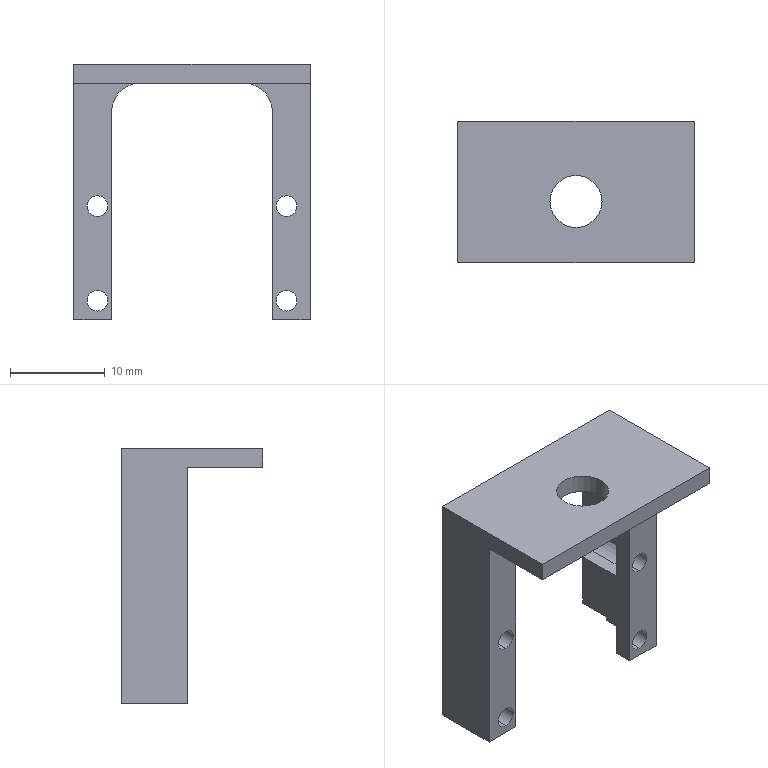Part | SolidWorks | features BaseBody 1 | 1 solid | 40 faces | box 25 x 15 x 27 mm | volume 1845 mm3 | plane 24 | cylinder 16 | commonest cylinder face diameters 2.2 x8 4 x4 5.5 x2 6 x2
STEP:
#1=CARTESIAN_POINT('',(9.75,-3.5,0.));
#2=VERTEX_POINT('',#1);
#3=CARTESIAN_POINT('',(15.25,-3.5,0.));
#4=VERTEX_POINT('',#3);
#5=CARTESIAN_POINT('',(12.5,-3.5,0.));
#6=DIRECTION('',(0.,0.,1.));
#7=DIRECTION('',(1.,0.,0.));
#8=AXIS2_PLACEMENT_3D('',#5,#6,#7);
#9=CIRCLE('',#8,2.75);
#10=EDGE_CURVE('',#2,#4,#9,.T.);
#11=ORIENTED_EDGE('',*,*,#10,.F.);
#12=CARTESIAN_POINT('',(9.75,-3.5,2.));
#13=VERTEX_POINT('',#12);
#14=CARTESIAN_POINT('',(9.75,-3.5,-13.));
#15=DIRECTION('',(0.,0.,1.));
#16=VECTOR('',#15,1000.);
#17=LINE('',#14,#16);
#18=EDGE_CURVE('',#2,#13,#17,.T.);
#19=ORIENTED_EDGE('',*,*,#18,.T.);
#20=CARTESIAN_POINT('',(15.25,-3.5,2.));
#21=VERTEX_POINT('',#20);
#22=CARTESIAN_POINT('',(12.5,-3.5,2.));
#23=DIRECTION('',(0.,0.,1.));
#24=DIRECTION('',(1.,0.,0.));
#25=AXIS2_PLACEMENT_3D('',#22,#23,#24);
#26=CIRCLE('',#25,2.75);
#27=EDGE_CURVE('',#13,#21,#26,.T.);
#28=ORIENTED_EDGE('',*,*,#27,.T.);
#29=CARTESIAN_POINT('',(15.25,-3.5,-13.));
#30=DIRECTION('',(0.,0.,1.));
#31=VECTOR('',#30,1000.);
#32=LINE('',#29,#31);
#33=EDGE_CURVE('',#4,#21,#32,.T.);
#34=ORIENTED_EDGE('',*,*,#33,.F.);
#35=EDGE_LOOP('',(#11,#19,#28,#34));
#36=FACE_OUTER_BOUND('',#35,.T.);
#37=CARTESIAN_POINT('',(12.5,-3.5,-13.));
#38=DIRECTION('',(0.,0.,1.));
#39=DIRECTION('',(1.,0.,0.));
#40=AXIS2_PLACEMENT_3D('',#37,#38,#39);
#41=CYLINDRICAL_SURFACE('',#40,2.75);
#42=ADVANCED_FACE('',(#36),#41,.F.);
#43=CARTESIAN_POINT('',(22.5,-2.,-21.9));
#44=VERTEX_POINT('',#43);
#45=CARTESIAN_POINT('',(22.5,-2.,-24.1));
#46=VERTEX_POINT('',#45);
#47=CARTESIAN_POINT('',(22.5,-2.,-23.));
#48=DIRECTION('',(0.,-1.,0.));
#49=DIRECTION('',(0.,0.,1.));
#50=AXIS2_PLACEMENT_3D('',#47,#48,#49);
#51=CIRCLE('',#50,1.1);
#52=EDGE_CURVE('',#44,#46,#51,.T.);
#53=ORIENTED_EDGE('',*,*,#52,.T.);
#54=CARTESIAN_POINT('',(22.5,0.,-24.1));
#55=VERTEX_POINT('',#54);
#56=CARTESIAN_POINT('',(22.5,-11.,-24.1));
#57=DIRECTION('',(0.,1.,0.));
#58=VECTOR('',#57,1000.);
#59=LINE('',#56,#58);
#60=EDGE_CURVE('',#46,#55,#59,.T.);
#61=ORIENTED_EDGE('',*,*,#60,.T.);
#62=CARTESIAN_POINT('',(22.5,0.,-21.9));
#63=VERTEX_POINT('',#62);
#64=CARTESIAN_POINT('',(22.5,0.,-23.));
#65=DIRECTION('',(0.,-1.,0.));
#66=DIRECTION('',(0.,0.,1.));
#67=AXIS2_PLACEMENT_3D('',#64,#65,#66);
#68=CIRCLE('',#67,1.1);
#69=EDGE_CURVE('',#63,#55,#68,.T.);
#70=ORIENTED_EDGE('',*,*,#69,.F.);
#71=CARTESIAN_POINT('',(22.5,-11.,-21.9));
#72=DIRECTION('',(0.,1.,0.));
#73=VECTOR('',#72,1000.);
#74=LINE('',#71,#73);
#75=EDGE_CURVE('',#44,#63,#74,.T.);
#76=ORIENTED_EDGE('',*,*,#75,.F.);
#77=EDGE_LOOP('',(#53,#61,#70,#76));
#78=FACE_OUTER_BOUND('',#77,.T.);
#79=CARTESIAN_POINT('',(22.5,-11.,-23.));
#80=DIRECTION('',(0.,1.,0.));
#81=DIRECTION('',(0.,0.,1.));
#82=AXIS2_PLACEMENT_3D('',#79,#80,#81);
#83=CYLINDRICAL_SURFACE('',#82,1.1);
#84=ADVANCED_FACE('',(#78),#83,.F.);
#85=CARTESIAN_POINT('',(22.5,-2.,-11.9));
#86=VERTEX_POINT('',#85);
#87=CARTESIAN_POINT('',(22.5,-2.,-14.1));
#88=VERTEX_POINT('',#87);
#89=CARTESIAN_POINT('',(22.5,-2.,-13.));
#90=DIRECTION('',(0.,-1.,0.));
#91=DIRECTION('',(0.,0.,1.));
#92=AXIS2_PLACEMENT_3D('',#89,#90,#91);
#93=CIRCLE('',#92,1.1);
#94=EDGE_CURVE('',#86,#88,#93,.T.);
#95=ORIENTED_EDGE('',*,*,#94,.T.);
#96=CARTESIAN_POINT('',(22.5,0.,-14.1));
#97=VERTEX_POINT('',#96);
#98=CARTESIAN_POINT('',(22.5,-11.,-14.1));
#99=DIRECTION('',(0.,1.,0.));
#100=VECTOR('',#99,1000.);
#101=LINE('',#98,#100);
#102=EDGE_CURVE('',#88,#97,#101,.T.);
#103=ORIENTED_EDGE('',*,*,#102,.T.);
#104=CARTESIAN_POINT('',(22.5,0.,-11.9));
#105=VERTEX_POINT('',#104);
#106=CARTESIAN_POINT('',(22.5,0.,-13.));
#107=DIRECTION('',(0.,-1.,0.));
#108=DIRECTION('',(0.,0.,1.));
#109=AXIS2_PLACEMENT_3D('',#106,#107,#108);
#110=CIRCLE('',#109,1.1);
#111=EDGE_CURVE('',#105,#97,#110,.T.);
#112=ORIENTED_EDGE('',*,*,#111,.F.);
#113=CARTESIAN_POINT('',(22.5,-11.,-11.9));
#114=DIRECTION('',(0.,1.,0.));
#115=VECTOR('',#114,1000.);
#116=LINE('',#113,#115);
#117=EDGE_CURVE('',#86,#105,#116,.T.);
#118=ORIENTED_EDGE('',*,*,#117,.F.);
#119=EDGE_LOOP('',(#95,#103,#112,#118));
#120=FACE_OUTER_BOUND('',#119,.T.);
#121=CARTESIAN_POINT('',(22.5,-11.,-13.));
#122=DIRECTION('',(0.,1.,0.));
#123=DIRECTION('',(0.,0.,1.));
#124=AXIS2_PLACEMENT_3D('',#121,#122,#123);
#125=CYLINDRICAL_SURFACE('',#124,1.1);
#126=ADVANCED_FACE('',(#120),#125,.F.);
#127=CARTESIAN_POINT('',(2.5,-2.,-11.9));
#128=VERTEX_POINT('',#127);
#129=CARTESIAN_POINT('',(2.5,-2.,-14.1));
#130=VERTEX_POINT('',#129);
#131=CARTESIAN_POINT('',(2.5,-2.,-13.));
#132=DIRECTION('',(0.,-1.,0.));
#133=DIRECTION('',(0.,0.,1.));
#134=AXIS2_PLACEMENT_3D('',#131,#132,#133);
#135=CIRCLE('',#134,1.1);
#136=EDGE_CURVE('',#128,#130,#135,.T.);
#137=ORIENTED_EDGE('',*,*,#136,.T.);
#138=CARTESIAN_POINT('',(2.5,0.,-14.1));
#139=VERTEX_POINT('',#138);
#140=CARTESIAN_POINT('',(2.5,-11.,-14.1));
#141=DIRECTION('',(0.,1.,0.));
#142=VECTOR('',#141,1000.);
#143=LINE('',#140,#142);
#144=EDGE_CURVE('',#130,#139,#143,.T.);
#145=ORIENTED_EDGE('',*,*,#144,.T.);
#146=CARTESIAN_POINT('',(2.5,0.,-11.9));
#147=VERTEX_POINT('',#146);
#148=CARTESIAN_POINT('',(2.5,0.,-13.));
#149=DIRECTION('',(0.,1.,0.));
#150=DIRECTION('',(0.,0.,1.));
#151=AXIS2_PLACEMENT_3D('',#148,#149,#150);
#152=CIRCLE('',#151,1.1);
#153=EDGE_CURVE('',#139,#147,#152,.T.);
#154=ORIENTED_EDGE('',*,*,#153,.T.);
#155=CARTESIAN_POINT('',(2.5,-11.,-11.9));
#156=DIRECTION('',(0.,1.,0.));
#157=VECTOR('',#156,1000.);
#158=LINE('',#155,#157);
#159=EDGE_CURVE('',#128,#147,#158,.T.);
#160=ORIENTED_EDGE('',*,*,#159,.F.);
#161=EDGE_LOOP('',(#137,#145,#154,#160));
#162=FACE_OUTER_BOUND('',#161,.T.);
#163=CARTESIAN_POINT('',(2.5,-11.,-13.));
#164=DIRECTION('',(0.,1.,0.));
#165=DIRECTION('',(0.,0.,1.));
#166=AXIS2_PLACEMENT_3D('',#163,#164,#165);
#167=CYLINDRICAL_SURFACE('',#166,1.1);
#168=ADVANCED_FACE('',(#162),#167,.F.);
#169=CARTESIAN_POINT('',(2.5,-2.,-21.9));
#170=VERTEX_POINT('',#169);
#171=CARTESIAN_POINT('',(2.5,-2.,-24.1));
#172=VERTEX_POINT('',#171);
#173=CARTESIAN_POINT('',(2.5,-2.,-23.));
#174=DIRECTION('',(0.,-1.,0.));
#175=DIRECTION('',(0.,0.,1.));
#176=AXIS2_PLACEMENT_3D('',#173,#174,#175);
#177=CIRCLE('',#176,1.1);
#178=EDGE_CURVE('',#170,#172,#177,.T.);
#179=ORIENTED_EDGE('',*,*,#178,.T.);
#180=CARTESIAN_POINT('',(2.5,0.,-24.1));
#181=VERTEX_POINT('',#180);
#182=CARTESIAN_POINT('',(2.5,-11.,-24.1));
#183=DIRECTION('',(0.,1.,0.));
#184=VECTOR('',#183,1000.);
#185=LINE('',#182,#184);
#186=EDGE_CURVE('',#172,#181,#185,.T.);
#187=ORIENTED_EDGE('',*,*,#186,.T.);
#188=CARTESIAN_POINT('',(2.5,0.,-21.9));
#189=VERTEX_POINT('',#188);
#190=CARTESIAN_POINT('',(2.5,0.,-23.));
#191=DIRECTION('',(0.,1.,0.));
#192=DIRECTION('',(0.,0.,1.));
#193=AXIS2_PLACEMENT_3D('',#190,#191,#192);
#194=CIRCLE('',#193,1.1);
#195=EDGE_CURVE('',#181,#189,#194,.T.);
#196=ORIENTED_EDGE('',*,*,#195,.T.);
#197=CARTESIAN_POINT('',(2.5,-11.,-21.9));
#198=DIRECTION('',(0.,1.,0.));
#199=VECTOR('',#198,1000.);
#200=LINE('',#197,#199);
#201=EDGE_CURVE('',#170,#189,#200,.T.);
#202=ORIENTED_EDGE('',*,*,#201,.F.);
#203=EDGE_LOOP('',(#179,#187,#196,#202));
#204=FACE_OUTER_BOUND('',#203,.T.);
#205=CARTESIAN_POINT('',(2.5,-11.,-23.));
#206=DIRECTION('',(0.,1.,0.));
#207=DIRECTION('',(0.,0.,1.));
#208=AXIS2_PLACEMENT_3D('',#205,#206,#207);
#209=CYLINDRICAL_SURFACE('',#208,1.1);
#210=ADVANCED_FACE('',(#204),#209,.F.);
#211=CARTESIAN_POINT('',(25.,5.,2.));
#212=VERTEX_POINT('',#211);
#213=CARTESIAN_POINT('',(25.,-10.,2.));
#214=VERTEX_POINT('',#213);
#215=CARTESIAN_POINT('',(25.,0.,2.));
#216=DIRECTION('',(0.,-1.,0.));
#217=VECTOR('',#216,1000.);
#218=LINE('',#215,#217);
#219=EDGE_CURVE('',#212,#214,#218,.T.);
#220=ORIENTED_EDGE('',*,*,#219,.F.);
#221=CARTESIAN_POINT('',(0.,5.,2.));
#222=VERTEX_POINT('',#221);
#223=CARTESIAN_POINT('',(0.,5.,2.));
#224=DIRECTION('',(1.,0.,0.));
#225=VECTOR('',#224,1000.);
#226=LINE('',#223,#225);
#227=EDGE_CURVE('',#222,#212,#226,.T.);
#228=ORIENTED_EDGE('',*,*,#227,.F.);
#229=CARTESIAN_POINT('',(0.,-10.,2.));
#230=VERTEX_POINT('',#229);
#231=CARTESIAN_POINT('',(0.,0.,2.));
#232=DIRECTION('',(0.,1.,0.));
#233=VECTOR('',#232,1000.);
#234=LINE('',#231,#233);
#235=EDGE_CURVE('',#230,#222,#234,.T.);
#236=ORIENTED_EDGE('',*,*,#235,.F.);
#237=CARTESIAN_POINT('',(0.,-10.,2.));
#238=DIRECTION('',(-1.,0.,0.));
#239=VECTOR('',#238,1000.);
#240=LINE('',#237,#239);
#241=EDGE_CURVE('',#214,#230,#240,.T.);
#242=ORIENTED_EDGE('',*,*,#241,.F.);
#243=EDGE_LOOP('',(#220,#228,#236,#242));
#244=FACE_OUTER_BOUND('',#243,.T.);
#245=CARTESIAN_POINT('',(12.5,-3.5,2.));
#246=DIRECTION('',(0.,0.,1.));
#247=DIRECTION('',(1.,0.,0.));
#248=AXIS2_PLACEMENT_3D('',#245,#246,#247);
#249=CIRCLE('',#248,2.75);
#250=EDGE_CURVE('',#21,#13,#249,.T.);
#251=ORIENTED_EDGE('',*,*,#250,.F.);
#252=ORIENTED_EDGE('',*,*,#27,.F.);
#253=EDGE_LOOP('',(#251,#252));
#254=FACE_BOUND('',#253,.T.);
#255=CARTESIAN_POINT('',(0.,0.,2.));
#256=DIRECTION('',(0.,0.,-1.));
#257=DIRECTION('',(-1.,0.,0.));
#258=AXIS2_PLACEMENT_3D('',#255,#256,#257);
#259=PLANE('',#258);
#260=ADVANCED_FACE('',(#244,#254),#259,.F.);
#261=CARTESIAN_POINT('',(25.,-10.,0.));
#262=VERTEX_POINT('',#261);
#263=CARTESIAN_POINT('',(25.,-10.,2.));
#264=DIRECTION('',(0.,0.,-1.));
#265=VECTOR('',#264,1000.);
#266=LINE('',#263,#265);
#267=EDGE_CURVE('',#214,#262,#266,.T.);
#268=ORIENTED_EDGE('',*,*,#267,.F.);
#269=ORIENTED_EDGE('',*,*,#241,.T.);
#270=CARTESIAN_POINT('',(0.,-10.,0.));
#271=VERTEX_POINT('',#270);
#272=CARTESIAN_POINT('',(0.,-10.,2.));
#273=DIRECTION('',(0.,0.,1.));
#274=VECTOR('',#273,1000.);
#275=LINE('',#272,#274);
#276=EDGE_CURVE('',#271,#230,#275,.T.);
#277=ORIENTED_EDGE('',*,*,#276,.F.);
#278=CARTESIAN_POINT('',(0.,-10.,0.));
#279=DIRECTION('',(-1.,0.,0.));
#280=VECTOR('',#279,1000.);
#281=LINE('',#278,#280);
#282=EDGE_CURVE('',#262,#271,#281,.T.);
#283=ORIENTED_EDGE('',*,*,#282,.F.);
#284=EDGE_LOOP('',(#268,#269,#277,#283));
#285=FACE_OUTER_BOUND('',#284,.T.);
#286=CARTESIAN_POINT('',(0.,-10.,2.));
#287=DIRECTION('',(0.,1.,0.));
#288=DIRECTION('',(0.,0.,1.));
#289=AXIS2_PLACEMENT_3D('',#286,#287,#288);
#290=PLANE('',#289);
#291=ADVANCED_FACE('',(#285),#290,.F.);
#292=ORIENTED_EDGE('',*,*,#219,.T.);
#293=ORIENTED_EDGE('',*,*,#267,.T.);
#294=CARTESIAN_POINT('',(25.,-2.,0.));
#295=VERTEX_POINT('',#294);
#296=CARTESIAN_POINT('',(25.,0.,0.));
#297=DIRECTION('',(0.,1.,0.));
#298=VECTOR('',#297,1000.);
#299=LINE('',#296,#298);
#300=EDGE_CURVE('',#262,#295,#299,.T.);
#301=ORIENTED_EDGE('',*,*,#300,.T.);
#302=CARTESIAN_POINT('',(25.,-2.,-25.));
#303=VERTEX_POINT('',#302);
#304=CARTESIAN_POINT('',(25.,-2.,2.));
#305=DIRECTION('',(0.,0.,-1.));
#306=VECTOR('',#305,1000.);
#307=LINE('',#304,#306);
#308=EDGE_CURVE('',#295,#303,#307,.T.);
#309=ORIENTED_EDGE('',*,*,#308,.T.);
#310=CARTESIAN_POINT('',(25.,5.,-25.));
#311=VERTEX_POINT('',#310);
#312=CARTESIAN_POINT('',(25.,0.,-25.));
#313=DIRECTION('',(0.,1.,0.));
#314=VECTOR('',#313,1000.);
#315=LINE('',#312,#314);
#316=EDGE_CURVE('',#303,#311,#315,.T.);
#317=ORIENTED_EDGE('',*,*,#316,.T.);
#318=CARTESIAN_POINT('',(25.,5.,2.));
#319=DIRECTION('',(0.,0.,1.));
#320=VECTOR('',#319,1000.);
#321=LINE('',#318,#320);
#322=EDGE_CURVE('',#311,#212,#321,.T.);
#323=ORIENTED_EDGE('',*,*,#322,.T.);
#324=EDGE_LOOP('',(#292,#293,#301,#309,#317,#323));
#325=FACE_OUTER_BOUND('',#324,.T.);
#326=CARTESIAN_POINT('',(25.,0.,2.));
#327=DIRECTION('',(1.,0.,0.));
#328=DIRECTION('',(0.,0.,-1.));
#329=AXIS2_PLACEMENT_3D('',#326,#327,#328);
#330=PLANE('',#329);
#331=ADVANCED_FACE('',(#325),#330,.T.);
#332=CARTESIAN_POINT('',(0.5,5.,-25.));
#333=VERTEX_POINT('',#332);
#334=CARTESIAN_POINT('',(0.5,5.,-23.));
#335=VERTEX_POINT('',#334);
#336=CARTESIAN_POINT('',(0.5,5.,0.));
#337=DIRECTION('',(0.,0.,1.));
#338=VECTOR('',#337,1000.);
#339=LINE('',#336,#338);
#340=EDGE_CURVE('',#333,#335,#339,.T.);
#341=ORIENTED_EDGE('',*,*,#340,.F.);
#342=CARTESIAN_POINT('',(0.,5.,-25.));
#343=VERTEX_POINT('',#342);
#344=CARTESIAN_POINT('',(0.,5.,-25.));
#345=DIRECTION('',(-1.,0.,0.));
#346=VECTOR('',#345,1000.);
#347=LINE('',#344,#346);
#348=EDGE_CURVE('',#333,#343,#347,.T.);
#349=ORIENTED_EDGE('',*,*,#348,.T.);
#350=CARTESIAN_POINT('',(0.,5.,0.));
#351=DIRECTION('',(0.,0.,-1.));
#352=VECTOR('',#351,1000.);
#353=LINE('',#350,#352);
#354=EDGE_CURVE('',#222,#343,#353,.T.);
#355=ORIENTED_EDGE('',*,*,#354,.F.);
#356=ORIENTED_EDGE('',*,*,#227,.T.);
#357=ORIENTED_EDGE('',*,*,#322,.F.);
#358=CARTESIAN_POINT('',(24.5,5.,-25.));
#359=VERTEX_POINT('',#358);
#360=CARTESIAN_POINT('',(0.,5.,-25.));
#361=DIRECTION('',(1.,0.,0.));
#362=VECTOR('',#361,1000.);
#363=LINE('',#360,#362);
#364=EDGE_CURVE('',#359,#311,#363,.T.);
#365=ORIENTED_EDGE('',*,*,#364,.F.);
#366=CARTESIAN_POINT('',(24.5,5.,-23.));
#367=VERTEX_POINT('',#366);
#368=CARTESIAN_POINT('',(24.5,5.,0.));
#369=DIRECTION('',(0.,0.,-1.));
#370=VECTOR('',#369,1000.);
#371=LINE('',#368,#370);
#372=EDGE_CURVE('',#367,#359,#371,.T.);
#373=ORIENTED_EDGE('',*,*,#372,.F.);
#374=CARTESIAN_POINT('',(22.5,5.,-21.));
#375=VERTEX_POINT('',#374);
#376=CARTESIAN_POINT('',(22.5,5.,-23.));
#377=DIRECTION('',(0.,1.,0.));
#378=DIRECTION('',(0.,0.,1.));
#379=AXIS2_PLACEMENT_3D('',#376,#377,#378);
#380=CIRCLE('',#379,2.);
#381=EDGE_CURVE('',#375,#367,#380,.T.);
#382=ORIENTED_EDGE('',*,*,#381,.F.);
#383=CARTESIAN_POINT('',(21.,5.,-21.));
#384=VERTEX_POINT('',#383);
#385=CARTESIAN_POINT('',(22.5,5.,-21.));
#386=DIRECTION('',(-1.,0.,0.));
#387=VECTOR('',#386,1000.);
#388=LINE('',#385,#387);
#389=EDGE_CURVE('',#375,#384,#388,.T.);
#390=ORIENTED_EDGE('',*,*,#389,.T.);
#391=CARTESIAN_POINT('',(21.,5.,-15.));
#392=VERTEX_POINT('',#391);
#393=CARTESIAN_POINT('',(21.,5.,0.));
#394=DIRECTION('',(0.,0.,-1.));
#395=VECTOR('',#394,1000.);
#396=LINE('',#393,#395);
#397=EDGE_CURVE('',#392,#384,#396,.T.);
#398=ORIENTED_EDGE('',*,*,#397,.F.);
#399=CARTESIAN_POINT('',(22.5,5.,-15.));
#400=VERTEX_POINT('',#399);
#401=CARTESIAN_POINT('',(22.5,5.,-15.));
#402=DIRECTION('',(1.,0.,0.));
#403=VECTOR('',#402,1000.);
#404=LINE('',#401,#403);
#405=EDGE_CURVE('',#392,#400,#404,.T.);
#406=ORIENTED_EDGE('',*,*,#405,.T.);
#407=CARTESIAN_POINT('',(22.5,5.,-11.));
#408=VERTEX_POINT('',#407);
#409=CARTESIAN_POINT('',(22.5,5.,-13.));
#410=DIRECTION('',(0.,1.,0.));
#411=DIRECTION('',(0.,0.,1.));
#412=AXIS2_PLACEMENT_3D('',#409,#410,#411);
#413=CIRCLE('',#412,2.);
#414=EDGE_CURVE('',#408,#400,#413,.T.);
#415=ORIENTED_EDGE('',*,*,#414,.F.);
#416=CARTESIAN_POINT('',(21.,5.,-11.));
#417=VERTEX_POINT('',#416);
#418=CARTESIAN_POINT('',(22.5,5.,-11.));
#419=DIRECTION('',(-1.,0.,0.));
#420=VECTOR('',#419,1000.);
#421=LINE('',#418,#420);
#422=EDGE_CURVE('',#408,#417,#421,.T.);
#423=ORIENTED_EDGE('',*,*,#422,.T.);
#424=CARTESIAN_POINT('',(21.,5.,-3.));
#425=VERTEX_POINT('',#424);
#426=CARTESIAN_POINT('',(21.,5.,0.));
#427=DIRECTION('',(0.,0.,-1.));
#428=VECTOR('',#427,1000.);
#429=LINE('',#426,#428);
#430=EDGE_CURVE('',#425,#417,#429,.T.);
#431=ORIENTED_EDGE('',*,*,#430,.F.);
#432=CARTESIAN_POINT('',(18.,5.,0.));
#433=VERTEX_POINT('',#432);
#434=CARTESIAN_POINT('',(18.,5.,-3.));
#435=DIRECTION('',(0.,1.,0.));
#436=DIRECTION('',(0.,0.,1.));
#437=AXIS2_PLACEMENT_3D('',#434,#435,#436);
#438=CIRCLE('',#437,3.);
#439=EDGE_CURVE('',#433,#425,#438,.T.);
#440=ORIENTED_EDGE('',*,*,#439,.F.);
#441=CARTESIAN_POINT('',(7.,5.,0.));
#442=VERTEX_POINT('',#441);
#443=CARTESIAN_POINT('',(0.,5.,0.));
#444=DIRECTION('',(1.,0.,0.));
#445=VECTOR('',#444,1000.);
#446=LINE('',#443,#445);
#447=EDGE_CURVE('',#442,#433,#446,.T.);
#448=ORIENTED_EDGE('',*,*,#447,.F.);
#449=CARTESIAN_POINT('',(4.,5.,-3.));
#450=VERTEX_POINT('',#449);
#451=CARTESIAN_POINT('',(7.,5.,-3.));
#452=DIRECTION('',(0.,1.,0.));
#453=DIRECTION('',(0.,0.,-1.));
#454=AXIS2_PLACEMENT_3D('',#451,#452,#453);
#455=CIRCLE('',#454,3.);
#456=EDGE_CURVE('',#450,#442,#455,.T.);
#457=ORIENTED_EDGE('',*,*,#456,.F.);
#458=CARTESIAN_POINT('',(4.,5.,-11.));
#459=VERTEX_POINT('',#458);
#460=CARTESIAN_POINT('',(4.,5.,0.));
#461=DIRECTION('',(0.,0.,1.));
#462=VECTOR('',#461,1000.);
#463=LINE('',#460,#462);
#464=EDGE_CURVE('',#459,#450,#463,.T.);
#465=ORIENTED_EDGE('',*,*,#464,.F.);
#466=CARTESIAN_POINT('',(2.5,5.,-11.));
#467=VERTEX_POINT('',#466);
#468=CARTESIAN_POINT('',(2.5,5.,-11.));
#469=DIRECTION('',(-1.,0.,0.));
#470=VECTOR('',#469,1000.);
#471=LINE('',#468,#470);
#472=EDGE_CURVE('',#459,#467,#471,.T.);
#473=ORIENTED_EDGE('',*,*,#472,.T.);
#474=CARTESIAN_POINT('',(2.5,5.,-15.));
#475=VERTEX_POINT('',#474);
#476=CARTESIAN_POINT('',(2.5,5.,-13.));
#477=DIRECTION('',(0.,1.,0.));
#478=DIRECTION('',(0.,0.,1.));
#479=AXIS2_PLACEMENT_3D('',#476,#477,#478);
#480=CIRCLE('',#479,2.);
#481=EDGE_CURVE('',#475,#467,#480,.T.);
#482=ORIENTED_EDGE('',*,*,#481,.F.);
#483=CARTESIAN_POINT('',(4.,5.,-15.));
#484=VERTEX_POINT('',#483);
#485=CARTESIAN_POINT('',(2.5,5.,-15.));
#486=DIRECTION('',(1.,0.,0.));
#487=VECTOR('',#486,1000.);
#488=LINE('',#485,#487);
#489=EDGE_CURVE('',#475,#484,#488,.T.);
#490=ORIENTED_EDGE('',*,*,#489,.T.);
#491=CARTESIAN_POINT('',(4.,5.,-21.));
#492=VERTEX_POINT('',#491);
#493=CARTESIAN_POINT('',(4.,5.,0.));
#494=DIRECTION('',(0.,0.,1.));
#495=VECTOR('',#494,1000.);
#496=LINE('',#493,#495);
#497=EDGE_CURVE('',#492,#484,#496,.T.);
#498=ORIENTED_EDGE('',*,*,#497,.F.);
#499=CARTESIAN_POINT('',(2.5,5.,-21.));
#500=VERTEX_POINT('',#499);
#501=CARTESIAN_POINT('',(2.5,5.,-21.));
#502=DIRECTION('',(-1.,0.,0.));
#503=VECTOR('',#502,1000.);
#504=LINE('',#501,#503);
#505=EDGE_CURVE('',#492,#500,#504,.T.);
#506=ORIENTED_EDGE('',*,*,#505,.T.);
#507=CARTESIAN_POINT('',(2.5,5.,-23.));
#508=DIRECTION('',(0.,1.,0.));
#509=DIRECTION('',(0.,0.,1.));
#510=AXIS2_PLACEMENT_3D('',#507,#508,#509);
#511=CIRCLE('',#510,2.);
#512=EDGE_CURVE('',#335,#500,#511,.T.);
#513=ORIENTED_EDGE('',*,*,#512,.F.);
#514=EDGE_LOOP('',(#341,#349,#355,#356,#357,#365,#373,#382,#390,#398,#406,#415,#423,#431,#440,#448,#457,#465,#473,#482,#490,#498,#506,#513));
#515=FACE_OUTER_BOUND('',#514,.T.);
#516=CARTESIAN_POINT('',(0.,5.,0.));
#517=DIRECTION('',(0.,-1.,0.));
#518=DIRECTION('',(0.,0.,-1.));
#519=AXIS2_PLACEMENT_3D('',#516,#517,#518);
#520=PLANE('',#519);
#521=ADVANCED_FACE('',(#515),#520,.F.);
#522=ORIENTED_EDGE('',*,*,#354,.T.);
#523=CARTESIAN_POINT('',(0.,-2.,-25.));
#524=VERTEX_POINT('',#523);
#525=CARTESIAN_POINT('',(0.,0.,-25.));
#526=DIRECTION('',(0.,1.,0.));
#527=VECTOR('',#526,1000.);
#528=LINE('',#525,#527);
#529=EDGE_CURVE('',#524,#343,#528,.T.);
#530=ORIENTED_EDGE('',*,*,#529,.F.);
#531=CARTESIAN_POINT('',(0.,-2.,0.));
#532=VERTEX_POINT('',#531);
#533=CARTESIAN_POINT('',(0.,-2.,2.));
#534=DIRECTION('',(0.,0.,-1.));
#535=VECTOR('',#534,1000.);
#536=LINE('',#533,#535);
#537=EDGE_CURVE('',#532,#524,#536,.T.);
#538=ORIENTED_EDGE('',*,*,#537,.F.);
#539=CARTESIAN_POINT('',(0.,0.,0.));
#540=DIRECTION('',(0.,1.,0.));
#541=VECTOR('',#540,1000.);
#542=LINE('',#539,#541);
#543=EDGE_CURVE('',#271,#532,#542,.T.);
#544=ORIENTED_EDGE('',*,*,#543,.F.);
#545=ORIENTED_EDGE('',*,*,#276,.T.);
#546=ORIENTED_EDGE('',*,*,#235,.T.);
#547=EDGE_LOOP('',(#522,#530,#538,#544,#545,#546));
#548=FACE_OUTER_BOUND('',#547,.T.);
#549=CARTESIAN_POINT('',(0.,0.,2.));
#550=DIRECTION('',(1.,0.,0.));
#551=DIRECTION('',(0.,1.,0.));
#552=AXIS2_PLACEMENT_3D('',#549,#550,#551);
#553=PLANE('',#552);
#554=ADVANCED_FACE('',(#548),#553,.F.);
#555=ORIENTED_EDGE('',*,*,#18,.F.);
#556=CARTESIAN_POINT('',(12.5,-3.5,0.));
#557=DIRECTION('',(0.,0.,1.));
#558=DIRECTION('',(1.,0.,0.));
#559=AXIS2_PLACEMENT_3D('',#556,#557,#558);
#560=CIRCLE('',#559,2.75);
#561=EDGE_CURVE('',#4,#2,#560,.T.);
#562=ORIENTED_EDGE('',*,*,#561,.F.);
#563=ORIENTED_EDGE('',*,*,#33,.T.);
#564=ORIENTED_EDGE('',*,*,#250,.T.);
#565=EDGE_LOOP('',(#555,#562,#563,#564));
#566=FACE_OUTER_BOUND('',#565,.T.);
#567=CARTESIAN_POINT('',(12.5,-3.5,-13.));
#568=DIRECTION('',(0.,0.,1.));
#569=DIRECTION('',(1.,0.,0.));
#570=AXIS2_PLACEMENT_3D('',#567,#568,#569);
#571=CYLINDRICAL_SURFACE('',#570,2.75);
#572=ADVANCED_FACE('',(#566),#571,.F.);
#573=ORIENTED_EDGE('',*,*,#282,.T.);
#574=ORIENTED_EDGE('',*,*,#543,.T.);
#575=CARTESIAN_POINT('',(7.,-2.,0.));
#576=VERTEX_POINT('',#575);
#577=CARTESIAN_POINT('',(0.,-2.,0.));
#578=DIRECTION('',(1.,0.,0.));
#579=VECTOR('',#578,1000.);
#580=LINE('',#577,#579);
#581=EDGE_CURVE('',#532,#576,#580,.T.);
#582=ORIENTED_EDGE('',*,*,#581,.T.);
#583=CARTESIAN_POINT('',(7.,0.,0.));
#584=DIRECTION('',(0.,1.,0.));
#585=VECTOR('',#584,1000.);
#586=LINE('',#583,#585);
#587=EDGE_CURVE('',#576,#442,#586,.T.);
#588=ORIENTED_EDGE('',*,*,#587,.T.);
#589=ORIENTED_EDGE('',*,*,#447,.T.);
#590=CARTESIAN_POINT('',(18.,-2.,0.));
#591=VERTEX_POINT('',#590);
#592=CARTESIAN_POINT('',(18.,0.,0.));
#593=DIRECTION('',(0.,-1.,0.));
#594=VECTOR('',#593,1000.);
#595=LINE('',#592,#594);
#596=EDGE_CURVE('',#433,#591,#595,.T.);
#597=ORIENTED_EDGE('',*,*,#596,.T.);
#598=CARTESIAN_POINT('',(0.,-2.,0.));
#599=DIRECTION('',(1.,0.,0.));
#600=VECTOR('',#599,1000.);
#601=LINE('',#598,#600);
#602=EDGE_CURVE('',#591,#295,#601,.T.);
#603=ORIENTED_EDGE('',*,*,#602,.T.);
#604=ORIENTED_EDGE('',*,*,#300,.F.);
#605=EDGE_LOOP('',(#573,#574,#582,#588,#589,#597,#603,#604));
#606=FACE_OUTER_BOUND('',#605,.T.);
#607=ORIENTED_EDGE('',*,*,#561,.T.);
#608=ORIENTED_EDGE('',*,*,#10,.T.);
#609=EDGE_LOOP('',(#607,#608));
#610=FACE_BOUND('',#609,.T.);
#611=CARTESIAN_POINT('',(0.,0.,0.));
#612=DIRECTION('',(0.,0.,-1.));
#613=DIRECTION('',(-1.,0.,0.));
#614=AXIS2_PLACEMENT_3D('',#611,#612,#613);
#615=PLANE('',#614);
#616=ADVANCED_FACE('',(#606,#610),#615,.T.);
#617=CARTESIAN_POINT('',(21.,-2.,-25.));
#618=VERTEX_POINT('',#617);
#619=CARTESIAN_POINT('',(21.,0.,-25.));
#620=VERTEX_POINT('',#619);
#621=CARTESIAN_POINT('',(21.,0.,-25.));
#622=DIRECTION('',(0.,1.,0.));
#623=VECTOR('',#622,1000.);
#624=LINE('',#621,#623);
#625=EDGE_CURVE('',#618,#620,#624,.T.);
#626=ORIENTED_EDGE('',*,*,#625,.T.);
#627=CARTESIAN_POINT('',(24.5,0.,-25.));
#628=VERTEX_POINT('',#627);
#629=CARTESIAN_POINT('',(0.,0.,-25.));
#630=DIRECTION('',(1.,0.,0.));
#631=VECTOR('',#630,1000.);
#632=LINE('',#629,#631);
#633=EDGE_CURVE('',#620,#628,#632,.T.);
#634=ORIENTED_EDGE('',*,*,#633,.T.);
#635=CARTESIAN_POINT('',(24.5,0.,-25.));
#636=DIRECTION('',(0.,1.,0.));
#637=VECTOR('',#636,1000.);
#638=LINE('',#635,#637);
#639=EDGE_CURVE('',#628,#359,#638,.T.);
#640=ORIENTED_EDGE('',*,*,#639,.T.);
#641=ORIENTED_EDGE('',*,*,#364,.T.);
#642=ORIENTED_EDGE('',*,*,#316,.F.);
#643=CARTESIAN_POINT('',(0.,-2.,-25.));
#644=DIRECTION('',(-1.,0.,0.));
#645=VECTOR('',#644,1000.);
#646=LINE('',#643,#645);
#647=EDGE_CURVE('',#303,#618,#646,.T.);
#648=ORIENTED_EDGE('',*,*,#647,.T.);
#649=EDGE_LOOP('',(#626,#634,#640,#641,#642,#648));
#650=FACE_OUTER_BOUND('',#649,.T.);
#651=CARTESIAN_POINT('',(0.,0.,-25.));
#652=DIRECTION('',(0.,0.,-1.));
#653=DIRECTION('',(-1.,0.,0.));
#654=AXIS2_PLACEMENT_3D('',#651,#652,#653);
#655=PLANE('',#654);
#656=ADVANCED_FACE('',(#650),#655,.T.);
#657=CARTESIAN_POINT('',(21.,-2.,-3.));
#658=VERTEX_POINT('',#657);
#659=CARTESIAN_POINT('',(18.,-2.,-3.));
#660=DIRECTION('',(0.,-1.,0.));
#661=DIRECTION('',(0.,0.,1.));
#662=AXIS2_PLACEMENT_3D('',#659,#660,#661);
#663=CIRCLE('',#662,3.);
#664=EDGE_CURVE('',#658,#591,#663,.T.);
#665=ORIENTED_EDGE('',*,*,#664,.F.);
#666=CARTESIAN_POINT('',(21.,-2.,-25.));
#667=DIRECTION('',(0.,0.,1.));
#668=VECTOR('',#667,1000.);
#669=LINE('',#666,#668);
#670=EDGE_CURVE('',#618,#658,#669,.T.);
#671=ORIENTED_EDGE('',*,*,#670,.F.);
#672=ORIENTED_EDGE('',*,*,#647,.F.);
#673=ORIENTED_EDGE('',*,*,#308,.F.);
#674=ORIENTED_EDGE('',*,*,#602,.F.);
#675=EDGE_LOOP('',(#665,#671,#672,#673,#674));
#676=FACE_OUTER_BOUND('',#675,.T.);
#677=ORIENTED_EDGE('',*,*,#52,.F.);
#678=CARTESIAN_POINT('',(22.5,-2.,-23.));
#679=DIRECTION('',(0.,-1.,0.));
#680=DIRECTION('',(0.,0.,1.));
#681=AXIS2_PLACEMENT_3D('',#678,#679,#680);
#682=CIRCLE('',#681,1.1);
#683=EDGE_CURVE('',#46,#44,#682,.T.);
#684=ORIENTED_EDGE('',*,*,#683,.F.);
#685=EDGE_LOOP('',(#677,#684));
#686=FACE_BOUND('',#685,.T.);
#687=ORIENTED_EDGE('',*,*,#94,.F.);
#688=CARTESIAN_POINT('',(22.5,-2.,-13.));
#689=DIRECTION('',(0.,-1.,0.));
#690=DIRECTION('',(0.,0.,1.));
#691=AXIS2_PLACEMENT_3D('',#688,#689,#690);
#692=CIRCLE('',#691,1.1);
#693=EDGE_CURVE('',#88,#86,#692,.T.);
#694=ORIENTED_EDGE('',*,*,#693,.F.);
#695=EDGE_LOOP('',(#687,#694));
#696=FACE_BOUND('',#695,.T.);
#697=CARTESIAN_POINT('',(25.,-2.,-25.));
#698=DIRECTION('',(0.,1.,0.));
#699=DIRECTION('',(0.,0.,1.));
#700=AXIS2_PLACEMENT_3D('',#697,#698,#699);
#701=PLANE('',#700);
#702=ADVANCED_FACE('',(#676,#686,#696),#701,.F.);
#703=CARTESIAN_POINT('',(2.5,0.,-21.));
#704=VERTEX_POINT('',#703);
#705=CARTESIAN_POINT('',(2.5,0.,-21.));
#706=DIRECTION('',(0.,1.,0.));
#707=VECTOR('',#706,1000.);
#708=LINE('',#705,#707);
#709=EDGE_CURVE('',#704,#500,#708,.T.);
#710=ORIENTED_EDGE('',*,*,#709,.F.);
#711=CARTESIAN_POINT('',(0.5,0.,-23.));
#712=VERTEX_POINT('',#711);
#713=CARTESIAN_POINT('',(2.5,0.,-23.));
#714=DIRECTION('',(0.,1.,0.));
#715=DIRECTION('',(0.,0.,1.));
#716=AXIS2_PLACEMENT_3D('',#713,#714,#715);
#717=CIRCLE('',#716,2.);
#718=EDGE_CURVE('',#712,#704,#717,.T.);
#719=ORIENTED_EDGE('',*,*,#718,.F.);
#720=CARTESIAN_POINT('',(0.5,0.,-23.));
#721=DIRECTION('',(0.,-1.,0.));
#722=VECTOR('',#721,1000.);
#723=LINE('',#720,#722);
#724=EDGE_CURVE('',#335,#712,#723,.T.);
#725=ORIENTED_EDGE('',*,*,#724,.F.);
#726=ORIENTED_EDGE('',*,*,#512,.T.);
#727=EDGE_LOOP('',(#710,#719,#725,#726));
#728=FACE_OUTER_BOUND('',#727,.T.);
#729=CARTESIAN_POINT('',(2.5,0.,-23.));
#730=DIRECTION('',(0.,1.,0.));
#731=DIRECTION('',(0.,0.,1.));
#732=AXIS2_PLACEMENT_3D('',#729,#730,#731);
#733=CYLINDRICAL_SURFACE('',#732,2.);
#734=ADVANCED_FACE('',(#728),#733,.F.);
#735=ORIENTED_EDGE('',*,*,#724,.T.);
#736=CARTESIAN_POINT('',(0.5,0.,-25.));
#737=VERTEX_POINT('',#736);
#738=CARTESIAN_POINT('',(0.5,0.,-23.));
#739=DIRECTION('',(0.,0.,1.));
#740=VECTOR('',#739,1000.);
#741=LINE('',#738,#740);
#742=EDGE_CURVE('',#737,#712,#741,.T.);
#743=ORIENTED_EDGE('',*,*,#742,.F.);
#744=CARTESIAN_POINT('',(0.5,0.,-25.));
#745=DIRECTION('',(0.,-1.,0.));
#746=VECTOR('',#745,1000.);
#747=LINE('',#744,#746);
#748=EDGE_CURVE('',#333,#737,#747,.T.);
#749=ORIENTED_EDGE('',*,*,#748,.F.);
#750=ORIENTED_EDGE('',*,*,#340,.T.);
#751=EDGE_LOOP('',(#735,#743,#749,#750));
#752=FACE_OUTER_BOUND('',#751,.T.);
#753=CARTESIAN_POINT('',(0.5,0.,-23.));
#754=DIRECTION('',(-1.,0.,0.));
#755=DIRECTION('',(0.,0.,1.));
#756=AXIS2_PLACEMENT_3D('',#753,#754,#755);
#757=PLANE('',#756);
#758=ADVANCED_FACE('',(#752),#757,.F.);
#759=ORIENTED_EDGE('',*,*,#639,.F.);
#760=CARTESIAN_POINT('',(24.5,0.,-23.));
#761=VERTEX_POINT('',#760);
#762=CARTESIAN_POINT('',(24.5,0.,-23.));
#763=DIRECTION('',(0.,0.,-1.));
#764=VECTOR('',#763,1000.);
#765=LINE('',#762,#764);
#766=EDGE_CURVE('',#761,#628,#765,.T.);
#767=ORIENTED_EDGE('',*,*,#766,.F.);
#768=CARTESIAN_POINT('',(24.5,0.,-23.));
#769=DIRECTION('',(0.,-1.,0.));
#770=VECTOR('',#769,1000.);
#771=LINE('',#768,#770);
#772=EDGE_CURVE('',#367,#761,#771,.T.);
#773=ORIENTED_EDGE('',*,*,#772,.F.);
#774=ORIENTED_EDGE('',*,*,#372,.T.);
#775=EDGE_LOOP('',(#759,#767,#773,#774));
#776=FACE_OUTER_BOUND('',#775,.T.);
#777=CARTESIAN_POINT('',(24.5,0.,-23.));
#778=DIRECTION('',(1.,0.,0.));
#779=DIRECTION('',(0.,0.,-1.));
#780=AXIS2_PLACEMENT_3D('',#777,#778,#779);
#781=PLANE('',#780);
#782=ADVANCED_FACE('',(#776),#781,.F.);
#783=ORIENTED_EDGE('',*,*,#772,.T.);
#784=CARTESIAN_POINT('',(22.5,0.,-21.));
#785=VERTEX_POINT('',#784);
#786=CARTESIAN_POINT('',(22.5,0.,-23.));
#787=DIRECTION('',(0.,1.,0.));
#788=DIRECTION('',(0.,0.,1.));
#789=AXIS2_PLACEMENT_3D('',#786,#787,#788);
#790=CIRCLE('',#789,2.);
#791=EDGE_CURVE('',#785,#761,#790,.T.);
#792=ORIENTED_EDGE('',*,*,#791,.F.);
#793=CARTESIAN_POINT('',(22.5,0.,-21.));
#794=DIRECTION('',(0.,-1.,0.));
#795=VECTOR('',#794,1000.);
#796=LINE('',#793,#795);
#797=EDGE_CURVE('',#375,#785,#796,.T.);
#798=ORIENTED_EDGE('',*,*,#797,.F.);
#799=ORIENTED_EDGE('',*,*,#381,.T.);
#800=EDGE_LOOP('',(#783,#792,#798,#799));
#801=FACE_OUTER_BOUND('',#800,.T.);
#802=CARTESIAN_POINT('',(22.5,0.,-23.));
#803=DIRECTION('',(0.,1.,0.));
#804=DIRECTION('',(0.,0.,1.));
#805=AXIS2_PLACEMENT_3D('',#802,#803,#804);
#806=CYLINDRICAL_SURFACE('',#805,2.);
#807=ADVANCED_FACE('',(#801),#806,.F.);
#808=CARTESIAN_POINT('',(21.,0.,-11.));
#809=VERTEX_POINT('',#808);
#810=CARTESIAN_POINT('',(21.,0.,-11.));
#811=DIRECTION('',(0.,1.,0.));
#812=VECTOR('',#811,1000.);
#813=LINE('',#810,#812);
#814=EDGE_CURVE('',#809,#417,#813,.T.);
#815=ORIENTED_EDGE('',*,*,#814,.F.);
#816=CARTESIAN_POINT('',(21.,0.,-15.));
#817=VERTEX_POINT('',#816);
#818=CARTESIAN_POINT('',(21.,0.,-25.));
#819=DIRECTION('',(0.,0.,1.));
#820=VECTOR('',#819,1000.);
#821=LINE('',#818,#820);
#822=EDGE_CURVE('',#817,#809,#821,.T.);
#823=ORIENTED_EDGE('',*,*,#822,.F.);
#824=CARTESIAN_POINT('',(21.,0.,-15.));
#825=DIRECTION('',(0.,-1.,0.));
#826=VECTOR('',#825,1000.);
#827=LINE('',#824,#826);
#828=EDGE_CURVE('',#392,#817,#827,.T.);
#829=ORIENTED_EDGE('',*,*,#828,.F.);
#830=ORIENTED_EDGE('',*,*,#397,.T.);
#831=CARTESIAN_POINT('',(21.,0.,-21.));
#832=VERTEX_POINT('',#831);
#833=CARTESIAN_POINT('',(21.,0.,-21.));
#834=DIRECTION('',(0.,1.,0.));
#835=VECTOR('',#834,1000.);
#836=LINE('',#833,#835);
#837=EDGE_CURVE('',#832,#384,#836,.T.);
#838=ORIENTED_EDGE('',*,*,#837,.F.);
#839=CARTESIAN_POINT('',(21.,0.,-25.));
#840=DIRECTION('',(0.,0.,1.));
#841=VECTOR('',#840,1000.);
#842=LINE('',#839,#841);
#843=EDGE_CURVE('',#620,#832,#842,.T.);
#844=ORIENTED_EDGE('',*,*,#843,.F.);
#845=ORIENTED_EDGE('',*,*,#625,.F.);
#846=ORIENTED_EDGE('',*,*,#670,.T.);
#847=CARTESIAN_POINT('',(21.,0.,-3.));
#848=DIRECTION('',(0.,-1.,0.));
#849=VECTOR('',#848,1000.);
#850=LINE('',#847,#849);
#851=EDGE_CURVE('',#425,#658,#850,.T.);
#852=ORIENTED_EDGE('',*,*,#851,.F.);
#853=ORIENTED_EDGE('',*,*,#430,.T.);
#854=EDGE_LOOP('',(#815,#823,#829,#830,#838,#844,#845,#846,#852,#853));
#855=FACE_OUTER_BOUND('',#854,.T.);
#856=CARTESIAN_POINT('',(21.,0.,-25.));
#857=DIRECTION('',(1.,0.,0.));
#858=DIRECTION('',(0.,0.,-1.));
#859=AXIS2_PLACEMENT_3D('',#856,#857,#858);
#860=PLANE('',#859);
#861=ADVANCED_FACE('',(#855),#860,.F.);
#862=CARTESIAN_POINT('',(22.5,0.,-15.));
#863=VERTEX_POINT('',#862);
#864=CARTESIAN_POINT('',(22.5,0.,-15.));
#865=DIRECTION('',(0.,1.,0.));
#866=VECTOR('',#865,1000.);
#867=LINE('',#864,#866);
#868=EDGE_CURVE('',#863,#400,#867,.T.);
#869=ORIENTED_EDGE('',*,*,#868,.F.);
#870=CARTESIAN_POINT('',(22.5,0.,-11.));
#871=VERTEX_POINT('',#870);
#872=CARTESIAN_POINT('',(22.5,0.,-13.));
#873=DIRECTION('',(0.,1.,0.));
#874=DIRECTION('',(0.,0.,1.));
#875=AXIS2_PLACEMENT_3D('',#872,#873,#874);
#876=CIRCLE('',#875,2.);
#877=EDGE_CURVE('',#871,#863,#876,.T.);
#878=ORIENTED_EDGE('',*,*,#877,.F.);
#879=CARTESIAN_POINT('',(22.5,0.,-11.));
#880=DIRECTION('',(0.,-1.,0.));
#881=VECTOR('',#880,1000.);
#882=LINE('',#879,#881);
#883=EDGE_CURVE('',#408,#871,#882,.T.);
#884=ORIENTED_EDGE('',*,*,#883,.F.);
#885=ORIENTED_EDGE('',*,*,#414,.T.);
#886=EDGE_LOOP('',(#869,#878,#884,#885));
#887=FACE_OUTER_BOUND('',#886,.T.);
#888=CARTESIAN_POINT('',(22.5,0.,-13.));
#889=DIRECTION('',(0.,1.,0.));
#890=DIRECTION('',(0.,0.,1.));
#891=AXIS2_PLACEMENT_3D('',#888,#889,#890);
#892=CYLINDRICAL_SURFACE('',#891,2.);
#893=ADVANCED_FACE('',(#887),#892,.F.);
#894=ORIENTED_EDGE('',*,*,#596,.F.);
#895=ORIENTED_EDGE('',*,*,#439,.T.);
#896=ORIENTED_EDGE('',*,*,#851,.T.);
#897=ORIENTED_EDGE('',*,*,#664,.T.);
#898=EDGE_LOOP('',(#894,#895,#896,#897));
#899=FACE_OUTER_BOUND('',#898,.T.);
#900=CARTESIAN_POINT('',(18.,0.,-3.));
#901=DIRECTION('',(0.,1.,0.));
#902=DIRECTION('',(0.,0.,1.));
#903=AXIS2_PLACEMENT_3D('',#900,#901,#902);
#904=CYLINDRICAL_SURFACE('',#903,3.);
#905=ADVANCED_FACE('',(#899),#904,.F.);
#906=ORIENTED_EDGE('',*,*,#587,.F.);
#907=CARTESIAN_POINT('',(4.,-2.,-3.));
#908=VERTEX_POINT('',#907);
#909=CARTESIAN_POINT('',(7.,-2.,-3.));
#910=DIRECTION('',(0.,1.,0.));
#911=DIRECTION('',(0.,0.,-1.));
#912=AXIS2_PLACEMENT_3D('',#909,#910,#911);
#913=CIRCLE('',#912,3.);
#914=EDGE_CURVE('',#908,#576,#913,.T.);
#915=ORIENTED_EDGE('',*,*,#914,.F.);
#916=CARTESIAN_POINT('',(4.,0.,-3.));
#917=DIRECTION('',(0.,-1.,0.));
#918=VECTOR('',#917,1000.);
#919=LINE('',#916,#918);
#920=EDGE_CURVE('',#450,#908,#919,.T.);
#921=ORIENTED_EDGE('',*,*,#920,.F.);
#922=ORIENTED_EDGE('',*,*,#456,.T.);
#923=EDGE_LOOP('',(#906,#915,#921,#922));
#924=FACE_OUTER_BOUND('',#923,.T.);
#925=CARTESIAN_POINT('',(7.,0.,-3.));
#926=DIRECTION('',(0.,-1.,0.));
#927=DIRECTION('',(0.,0.,-1.));
#928=AXIS2_PLACEMENT_3D('',#925,#926,#927);
#929=CYLINDRICAL_SURFACE('',#928,3.);
#930=ADVANCED_FACE('',(#924),#929,.F.);
#931=CARTESIAN_POINT('',(4.,0.,-21.));
#932=VERTEX_POINT('',#931);
#933=CARTESIAN_POINT('',(4.,0.,-21.));
#934=DIRECTION('',(0.,-1.,0.));
#935=VECTOR('',#934,1000.);
#936=LINE('',#933,#935);
#937=EDGE_CURVE('',#492,#932,#936,.T.);
#938=ORIENTED_EDGE('',*,*,#937,.F.);
#939=ORIENTED_EDGE('',*,*,#497,.T.);
#940=CARTESIAN_POINT('',(4.,0.,-15.));
#941=VERTEX_POINT('',#940);
#942=CARTESIAN_POINT('',(4.,0.,-15.));
#943=DIRECTION('',(0.,1.,0.));
#944=VECTOR('',#943,1000.);
#945=LINE('',#942,#944);
#946=EDGE_CURVE('',#941,#484,#945,.T.);
#947=ORIENTED_EDGE('',*,*,#946,.F.);
#948=CARTESIAN_POINT('',(4.,0.,-11.));
#949=VERTEX_POINT('',#948);
#950=CARTESIAN_POINT('',(4.,0.,-25.));
#951=DIRECTION('',(0.,0.,-1.));
#952=VECTOR('',#951,1000.);
#953=LINE('',#950,#952);
#954=EDGE_CURVE('',#949,#941,#953,.T.);
#955=ORIENTED_EDGE('',*,*,#954,.F.);
#956=CARTESIAN_POINT('',(4.,0.,-11.));
#957=DIRECTION('',(0.,-1.,0.));
#958=VECTOR('',#957,1000.);
#959=LINE('',#956,#958);
#960=EDGE_CURVE('',#459,#949,#959,.T.);
#961=ORIENTED_EDGE('',*,*,#960,.F.);
#962=ORIENTED_EDGE('',*,*,#464,.T.);
#963=ORIENTED_EDGE('',*,*,#920,.T.);
#964=CARTESIAN_POINT('',(4.,-2.,-25.));
#965=VERTEX_POINT('',#964);
#966=CARTESIAN_POINT('',(4.,-2.,-25.));
#967=DIRECTION('',(0.,0.,1.));
#968=VECTOR('',#967,1000.);
#969=LINE('',#966,#968);
#970=EDGE_CURVE('',#965,#908,#969,.T.);
#971=ORIENTED_EDGE('',*,*,#970,.F.);
#972=CARTESIAN_POINT('',(4.,0.,-25.));
#973=VERTEX_POINT('',#972);
#974=CARTESIAN_POINT('',(4.,0.,-25.));
#975=DIRECTION('',(0.,-1.,0.));
#976=VECTOR('',#975,1000.);
#977=LINE('',#974,#976);
#978=EDGE_CURVE('',#973,#965,#977,.T.);
#979=ORIENTED_EDGE('',*,*,#978,.F.);
#980=CARTESIAN_POINT('',(4.,0.,-25.));
#981=DIRECTION('',(0.,0.,-1.));
#982=VECTOR('',#981,1000.);
#983=LINE('',#980,#982);
#984=EDGE_CURVE('',#932,#973,#983,.T.);
#985=ORIENTED_EDGE('',*,*,#984,.F.);
#986=EDGE_LOOP('',(#938,#939,#947,#955,#961,#962,#963,#971,#979,#985));
#987=FACE_OUTER_BOUND('',#986,.T.);
#988=CARTESIAN_POINT('',(4.,0.,-25.));
#989=DIRECTION('',(-1.,0.,0.));
#990=DIRECTION('',(0.,0.,1.));
#991=AXIS2_PLACEMENT_3D('',#988,#989,#990);
#992=PLANE('',#991);
#993=ADVANCED_FACE('',(#987),#992,.F.);
#994=CARTESIAN_POINT('',(2.5,0.,-11.));
#995=VERTEX_POINT('',#994);
#996=CARTESIAN_POINT('',(2.5,0.,-11.));
#997=DIRECTION('',(0.,1.,0.));
#998=VECTOR('',#997,1000.);
#999=LINE('',#996,#998);
#1000=EDGE_CURVE('',#995,#467,#999,.T.);
#1001=ORIENTED_EDGE('',*,*,#1000,.F.);
#1002=CARTESIAN_POINT('',(2.5,0.,-15.));
#1003=VERTEX_POINT('',#1002);
#1004=CARTESIAN_POINT('',(2.5,0.,-13.));
#1005=DIRECTION('',(0.,1.,0.));
#1006=DIRECTION('',(0.,0.,1.));
#1007=AXIS2_PLACEMENT_3D('',#1004,#1005,#1006);
#1008=CIRCLE('',#1007,2.);
#1009=EDGE_CURVE('',#1003,#995,#1008,.T.);
#1010=ORIENTED_EDGE('',*,*,#1009,.F.);
#1011=CARTESIAN_POINT('',(2.5,0.,-15.));
#1012=DIRECTION('',(0.,-1.,0.));
#1013=VECTOR('',#1012,1000.);
#1014=LINE('',#1011,#1013);
#1015=EDGE_CURVE('',#475,#1003,#1014,.T.);
#1016=ORIENTED_EDGE('',*,*,#1015,.F.);
#1017=ORIENTED_EDGE('',*,*,#481,.T.);
#1018=EDGE_LOOP('',(#1001,#1010,#1016,#1017));
#1019=FACE_OUTER_BOUND('',#1018,.T.);
#1020=CARTESIAN_POINT('',(2.5,0.,-13.));
#1021=DIRECTION('',(0.,1.,0.));
#1022=DIRECTION('',(0.,0.,1.));
#1023=AXIS2_PLACEMENT_3D('',#1020,#1021,#1022);
#1024=CYLINDRICAL_SURFACE('',#1023,2.);
#1025=ADVANCED_FACE('',(#1019),#1024,.F.);
#1026=ORIENTED_EDGE('',*,*,#748,.T.);
#1027=CARTESIAN_POINT('',(0.,0.,-25.));
#1028=DIRECTION('',(-1.,0.,0.));
#1029=VECTOR('',#1028,1000.);
#1030=LINE('',#1027,#1029);
#1031=EDGE_CURVE('',#973,#737,#1030,.T.);
#1032=ORIENTED_EDGE('',*,*,#1031,.F.);
#1033=ORIENTED_EDGE('',*,*,#978,.T.);
#1034=CARTESIAN_POINT('',(0.,-2.,-25.));
#1035=DIRECTION('',(1.,0.,0.));
#1036=VECTOR('',#1035,1000.);
#1037=LINE('',#1034,#1036);
#1038=EDGE_CURVE('',#524,#965,#1037,.T.);
#1039=ORIENTED_EDGE('',*,*,#1038,.F.);
#1040=ORIENTED_EDGE('',*,*,#529,.T.);
#1041=ORIENTED_EDGE('',*,*,#348,.F.);
#1042=EDGE_LOOP('',(#1026,#1032,#1033,#1039,#1040,#1041));
#1043=FACE_OUTER_BOUND('',#1042,.T.);
#1044=CARTESIAN_POINT('',(0.,0.,-25.));
#1045=DIRECTION('',(0.,0.,1.));
#1046=DIRECTION('',(1.,0.,0.));
#1047=AXIS2_PLACEMENT_3D('',#1044,#1045,#1046);
#1048=PLANE('',#1047);
#1049=ADVANCED_FACE('',(#1043),#1048,.F.);
#1050=ORIENTED_EDGE('',*,*,#537,.T.);
#1051=ORIENTED_EDGE('',*,*,#1038,.T.);
#1052=ORIENTED_EDGE('',*,*,#970,.T.);
#1053=ORIENTED_EDGE('',*,*,#914,.T.);
#1054=ORIENTED_EDGE('',*,*,#581,.F.);
#1055=EDGE_LOOP('',(#1050,#1051,#1052,#1053,#1054));
#1056=FACE_OUTER_BOUND('',#1055,.T.);
#1057=ORIENTED_EDGE('',*,*,#136,.F.);
#1058=CARTESIAN_POINT('',(2.5,-2.,-13.));
#1059=DIRECTION('',(0.,-1.,0.));
#1060=DIRECTION('',(0.,0.,1.));
#1061=AXIS2_PLACEMENT_3D('',#1058,#1059,#1060);
#1062=CIRCLE('',#1061,1.1);
#1063=EDGE_CURVE('',#130,#128,#1062,.T.);
#1064=ORIENTED_EDGE('',*,*,#1063,.F.);
#1065=EDGE_LOOP('',(#1057,#1064));
#1066=FACE_BOUND('',#1065,.T.);
#1067=ORIENTED_EDGE('',*,*,#178,.F.);
#1068=CARTESIAN_POINT('',(2.5,-2.,-23.));
#1069=DIRECTION('',(0.,-1.,0.));
#1070=DIRECTION('',(0.,0.,1.));
#1071=AXIS2_PLACEMENT_3D('',#1068,#1069,#1070);
#1072=CIRCLE('',#1071,1.1);
#1073=EDGE_CURVE('',#172,#170,#1072,.T.);
#1074=ORIENTED_EDGE('',*,*,#1073,.F.);
#1075=EDGE_LOOP('',(#1067,#1074));
#1076=FACE_BOUND('',#1075,.T.);
#1077=CARTESIAN_POINT('',(0.,-2.,-25.));
#1078=DIRECTION('',(0.,1.,0.));
#1079=DIRECTION('',(-1.,0.,0.));
#1080=AXIS2_PLACEMENT_3D('',#1077,#1078,#1079);
#1081=PLANE('',#1080);
#1082=ADVANCED_FACE('',(#1056,#1066,#1076),#1081,.F.);
#1083=ORIENTED_EDGE('',*,*,#69,.T.);
#1084=CARTESIAN_POINT('',(22.5,0.,-23.));
#1085=DIRECTION('',(0.,-1.,0.));
#1086=DIRECTION('',(0.,0.,1.));
#1087=AXIS2_PLACEMENT_3D('',#1084,#1085,#1086);
#1088=CIRCLE('',#1087,1.1);
#1089=EDGE_CURVE('',#55,#63,#1088,.T.);
#1090=ORIENTED_EDGE('',*,*,#1089,.T.);
#1091=EDGE_LOOP('',(#1083,#1090));
#1092=FACE_BOUND('',#1091,.T.);
#1093=ORIENTED_EDGE('',*,*,#843,.T.);
#1094=CARTESIAN_POINT('',(22.5,0.,-21.));
#1095=DIRECTION('',(1.,0.,0.));
#1096=VECTOR('',#1095,1000.);
#1097=LINE('',#1094,#1096);
#1098=EDGE_CURVE('',#832,#785,#1097,.T.);
#1099=ORIENTED_EDGE('',*,*,#1098,.T.);
#1100=ORIENTED_EDGE('',*,*,#791,.T.);
#1101=ORIENTED_EDGE('',*,*,#766,.T.);
#1102=ORIENTED_EDGE('',*,*,#633,.F.);
#1103=EDGE_LOOP('',(#1093,#1099,#1100,#1101,#1102));
#1104=FACE_OUTER_BOUND('',#1103,.T.);
#1105=CARTESIAN_POINT('',(22.5,0.,-23.));
#1106=DIRECTION('',(0.,1.,0.));
#1107=DIRECTION('',(0.,0.,1.));
#1108=AXIS2_PLACEMENT_3D('',#1105,#1106,#1107);
#1109=PLANE('',#1108);
#1110=ADVANCED_FACE('',(#1092,#1104),#1109,.T.);
#1111=ORIENTED_EDGE('',*,*,#60,.F.);
#1112=ORIENTED_EDGE('',*,*,#683,.T.);
#1113=ORIENTED_EDGE('',*,*,#75,.T.);
#1114=ORIENTED_EDGE('',*,*,#1089,.F.);
#1115=EDGE_LOOP('',(#1111,#1112,#1113,#1114));
#1116=FACE_OUTER_BOUND('',#1115,.T.);
#1117=CARTESIAN_POINT('',(22.5,-11.,-23.));
#1118=DIRECTION('',(0.,1.,0.));
#1119=DIRECTION('',(0.,0.,1.));
#1120=AXIS2_PLACEMENT_3D('',#1117,#1118,#1119);
#1121=CYLINDRICAL_SURFACE('',#1120,1.1);
#1122=ADVANCED_FACE('',(#1116),#1121,.F.);
#1123=ORIENTED_EDGE('',*,*,#102,.F.);
#1124=ORIENTED_EDGE('',*,*,#693,.T.);
#1125=ORIENTED_EDGE('',*,*,#117,.T.);
#1126=CARTESIAN_POINT('',(22.5,0.,-13.));
#1127=DIRECTION('',(0.,-1.,0.));
#1128=DIRECTION('',(0.,0.,1.));
#1129=AXIS2_PLACEMENT_3D('',#1126,#1127,#1128);
#1130=CIRCLE('',#1129,1.1);
#1131=EDGE_CURVE('',#97,#105,#1130,.T.);
#1132=ORIENTED_EDGE('',*,*,#1131,.F.);
#1133=EDGE_LOOP('',(#1123,#1124,#1125,#1132));
#1134=FACE_OUTER_BOUND('',#1133,.T.);
#1135=CARTESIAN_POINT('',(22.5,-11.,-13.));
#1136=DIRECTION('',(0.,1.,0.));
#1137=DIRECTION('',(0.,0.,1.));
#1138=AXIS2_PLACEMENT_3D('',#1135,#1136,#1137);
#1139=CYLINDRICAL_SURFACE('',#1138,1.1);
#1140=ADVANCED_FACE('',(#1134),#1139,.F.);
#1141=ORIENTED_EDGE('',*,*,#937,.T.);
#1142=CARTESIAN_POINT('',(2.5,0.,-21.));
#1143=DIRECTION('',(1.,0.,0.));
#1144=VECTOR('',#1143,1000.);
#1145=LINE('',#1142,#1144);
#1146=EDGE_CURVE('',#704,#932,#1145,.T.);
#1147=ORIENTED_EDGE('',*,*,#1146,.F.);
#1148=ORIENTED_EDGE('',*,*,#709,.T.);
#1149=ORIENTED_EDGE('',*,*,#505,.F.);
#1150=EDGE_LOOP('',(#1141,#1147,#1148,#1149));
#1151=FACE_OUTER_BOUND('',#1150,.T.);
#1152=CARTESIAN_POINT('',(2.5,0.,-21.));
#1153=DIRECTION('',(0.,0.,1.));
#1154=DIRECTION('',(1.,0.,0.));
#1155=AXIS2_PLACEMENT_3D('',#1152,#1153,#1154);
#1156=PLANE('',#1155);
#1157=ADVANCED_FACE('',(#1151),#1156,.F.);
#1158=CARTESIAN_POINT('',(2.5,0.,-23.));
#1159=DIRECTION('',(0.,1.,0.));
#1160=DIRECTION('',(0.,0.,1.));
#1161=AXIS2_PLACEMENT_3D('',#1158,#1159,#1160);
#1162=CIRCLE('',#1161,1.1);
#1163=EDGE_CURVE('',#189,#181,#1162,.T.);
#1164=ORIENTED_EDGE('',*,*,#1163,.F.);
#1165=ORIENTED_EDGE('',*,*,#195,.F.);
#1166=EDGE_LOOP('',(#1164,#1165));
#1167=FACE_BOUND('',#1166,.T.);
#1168=ORIENTED_EDGE('',*,*,#1146,.T.);
#1169=ORIENTED_EDGE('',*,*,#984,.T.);
#1170=ORIENTED_EDGE('',*,*,#1031,.T.);
#1171=ORIENTED_EDGE('',*,*,#742,.T.);
#1172=ORIENTED_EDGE('',*,*,#718,.T.);
#1173=EDGE_LOOP('',(#1168,#1169,#1170,#1171,#1172));
#1174=FACE_OUTER_BOUND('',#1173,.T.);
#1175=CARTESIAN_POINT('',(2.5,0.,-23.));
#1176=DIRECTION('',(0.,-1.,0.));
#1177=DIRECTION('',(0.,0.,-1.));
#1178=AXIS2_PLACEMENT_3D('',#1175,#1176,#1177);
#1179=PLANE('',#1178);
#1180=ADVANCED_FACE('',(#1167,#1174),#1179,.F.);
#1181=ORIENTED_EDGE('',*,*,#797,.T.);
#1182=ORIENTED_EDGE('',*,*,#1098,.F.);
#1183=ORIENTED_EDGE('',*,*,#837,.T.);
#1184=ORIENTED_EDGE('',*,*,#389,.F.);
#1185=EDGE_LOOP('',(#1181,#1182,#1183,#1184));
#1186=FACE_OUTER_BOUND('',#1185,.T.);
#1187=CARTESIAN_POINT('',(22.5,0.,-21.));
#1188=DIRECTION('',(0.,0.,1.));
#1189=DIRECTION('',(1.,0.,0.));
#1190=AXIS2_PLACEMENT_3D('',#1187,#1188,#1189);
#1191=PLANE('',#1190);
#1192=ADVANCED_FACE('',(#1186),#1191,.F.);
#1193=ORIENTED_EDGE('',*,*,#883,.T.);
#1194=CARTESIAN_POINT('',(22.5,0.,-11.));
#1195=DIRECTION('',(1.,0.,0.));
#1196=VECTOR('',#1195,1000.);
#1197=LINE('',#1194,#1196);
#1198=EDGE_CURVE('',#809,#871,#1197,.T.);
#1199=ORIENTED_EDGE('',*,*,#1198,.F.);
#1200=ORIENTED_EDGE('',*,*,#814,.T.);
#1201=ORIENTED_EDGE('',*,*,#422,.F.);
#1202=EDGE_LOOP('',(#1193,#1199,#1200,#1201));
#1203=FACE_OUTER_BOUND('',#1202,.T.);
#1204=CARTESIAN_POINT('',(22.5,0.,-11.));
#1205=DIRECTION('',(0.,0.,1.));
#1206=DIRECTION('',(1.,0.,0.));
#1207=AXIS2_PLACEMENT_3D('',#1204,#1205,#1206);
#1208=PLANE('',#1207);
#1209=ADVANCED_FACE('',(#1203),#1208,.F.);
#1210=ORIENTED_EDGE('',*,*,#111,.T.);
#1211=ORIENTED_EDGE('',*,*,#1131,.T.);
#1212=EDGE_LOOP('',(#1210,#1211));
#1213=FACE_BOUND('',#1212,.T.);
#1214=ORIENTED_EDGE('',*,*,#822,.T.);
#1215=ORIENTED_EDGE('',*,*,#1198,.T.);
#1216=ORIENTED_EDGE('',*,*,#877,.T.);
#1217=CARTESIAN_POINT('',(22.5,0.,-15.));
#1218=DIRECTION('',(-1.,0.,0.));
#1219=VECTOR('',#1218,1000.);
#1220=LINE('',#1217,#1219);
#1221=EDGE_CURVE('',#863,#817,#1220,.T.);
#1222=ORIENTED_EDGE('',*,*,#1221,.T.);
#1223=EDGE_LOOP('',(#1214,#1215,#1216,#1222));
#1224=FACE_OUTER_BOUND('',#1223,.T.);
#1225=CARTESIAN_POINT('',(22.5,0.,-13.));
#1226=DIRECTION('',(0.,1.,0.));
#1227=DIRECTION('',(0.,0.,1.));
#1228=AXIS2_PLACEMENT_3D('',#1225,#1226,#1227);
#1229=PLANE('',#1228);
#1230=ADVANCED_FACE('',(#1213,#1224),#1229,.T.);
#1231=ORIENTED_EDGE('',*,*,#828,.T.);
#1232=ORIENTED_EDGE('',*,*,#1221,.F.);
#1233=ORIENTED_EDGE('',*,*,#868,.T.);
#1234=ORIENTED_EDGE('',*,*,#405,.F.);
#1235=EDGE_LOOP('',(#1231,#1232,#1233,#1234));
#1236=FACE_OUTER_BOUND('',#1235,.T.);
#1237=CARTESIAN_POINT('',(22.5,0.,-15.));
#1238=DIRECTION('',(0.,0.,-1.));
#1239=DIRECTION('',(-1.,0.,0.));
#1240=AXIS2_PLACEMENT_3D('',#1237,#1238,#1239);
#1241=PLANE('',#1240);
#1242=ADVANCED_FACE('',(#1236),#1241,.F.);
#1243=ORIENTED_EDGE('',*,*,#1015,.T.);
#1244=CARTESIAN_POINT('',(2.5,0.,-15.));
#1245=DIRECTION('',(-1.,0.,0.));
#1246=VECTOR('',#1245,1000.);
#1247=LINE('',#1244,#1246);
#1248=EDGE_CURVE('',#941,#1003,#1247,.T.);
#1249=ORIENTED_EDGE('',*,*,#1248,.F.);
#1250=ORIENTED_EDGE('',*,*,#946,.T.);
#1251=ORIENTED_EDGE('',*,*,#489,.F.);
#1252=EDGE_LOOP('',(#1243,#1249,#1250,#1251));
#1253=FACE_OUTER_BOUND('',#1252,.T.);
#1254=CARTESIAN_POINT('',(2.5,0.,-15.));
#1255=DIRECTION('',(0.,0.,-1.));
#1256=DIRECTION('',(-1.,0.,0.));
#1257=AXIS2_PLACEMENT_3D('',#1254,#1255,#1256);
#1258=PLANE('',#1257);
#1259=ADVANCED_FACE('',(#1253),#1258,.F.);
#1260=CARTESIAN_POINT('',(2.5,0.,-13.));
#1261=DIRECTION('',(0.,1.,0.));
#1262=DIRECTION('',(0.,0.,1.));
#1263=AXIS2_PLACEMENT_3D('',#1260,#1261,#1262);
#1264=CIRCLE('',#1263,1.1);
#1265=EDGE_CURVE('',#147,#139,#1264,.T.);
#1266=ORIENTED_EDGE('',*,*,#1265,.F.);
#1267=ORIENTED_EDGE('',*,*,#153,.F.);
#1268=EDGE_LOOP('',(#1266,#1267));
#1269=FACE_BOUND('',#1268,.T.);
#1270=CARTESIAN_POINT('',(2.5,0.,-11.));
#1271=DIRECTION('',(-1.,0.,0.));
#1272=VECTOR('',#1271,1000.);
#1273=LINE('',#1270,#1272);
#1274=EDGE_CURVE('',#949,#995,#1273,.T.);
#1275=ORIENTED_EDGE('',*,*,#1274,.F.);
#1276=ORIENTED_EDGE('',*,*,#954,.T.);
#1277=ORIENTED_EDGE('',*,*,#1248,.T.);
#1278=ORIENTED_EDGE('',*,*,#1009,.T.);
#1279=EDGE_LOOP('',(#1275,#1276,#1277,#1278));
#1280=FACE_OUTER_BOUND('',#1279,.T.);
#1281=CARTESIAN_POINT('',(2.5,0.,-13.));
#1282=DIRECTION('',(0.,-1.,0.));
#1283=DIRECTION('',(0.,0.,-1.));
#1284=AXIS2_PLACEMENT_3D('',#1281,#1282,#1283);
#1285=PLANE('',#1284);
#1286=ADVANCED_FACE('',(#1269,#1280),#1285,.F.);
#1287=ORIENTED_EDGE('',*,*,#960,.T.);
#1288=ORIENTED_EDGE('',*,*,#1274,.T.);
#1289=ORIENTED_EDGE('',*,*,#1000,.T.);
#1290=ORIENTED_EDGE('',*,*,#472,.F.);
#1291=EDGE_LOOP('',(#1287,#1288,#1289,#1290));
#1292=FACE_OUTER_BOUND('',#1291,.T.);
#1293=CARTESIAN_POINT('',(2.5,0.,-11.));
#1294=DIRECTION('',(0.,0.,1.));
#1295=DIRECTION('',(1.,0.,0.));
#1296=AXIS2_PLACEMENT_3D('',#1293,#1294,#1295);
#1297=PLANE('',#1296);
#1298=ADVANCED_FACE('',(#1292),#1297,.F.);
#1299=ORIENTED_EDGE('',*,*,#144,.F.);
#1300=ORIENTED_EDGE('',*,*,#1063,.T.);
#1301=ORIENTED_EDGE('',*,*,#159,.T.);
#1302=ORIENTED_EDGE('',*,*,#1265,.T.);
#1303=EDGE_LOOP('',(#1299,#1300,#1301,#1302));
#1304=FACE_OUTER_BOUND('',#1303,.T.);
#1305=CARTESIAN_POINT('',(2.5,-11.,-13.));
#1306=DIRECTION('',(0.,1.,0.));
#1307=DIRECTION('',(0.,0.,1.));
#1308=AXIS2_PLACEMENT_3D('',#1305,#1306,#1307);
#1309=CYLINDRICAL_SURFACE('',#1308,1.1);
#1310=ADVANCED_FACE('',(#1304),#1309,.F.);
#1311=ORIENTED_EDGE('',*,*,#186,.F.);
#1312=ORIENTED_EDGE('',*,*,#1073,.T.);
#1313=ORIENTED_EDGE('',*,*,#201,.T.);
#1314=ORIENTED_EDGE('',*,*,#1163,.T.);
#1315=EDGE_LOOP('',(#1311,#1312,#1313,#1314));
#1316=FACE_OUTER_BOUND('',#1315,.T.);
#1317=CARTESIAN_POINT('',(2.5,-11.,-23.));
#1318=DIRECTION('',(0.,1.,0.));
#1319=DIRECTION('',(0.,0.,1.));
#1320=AXIS2_PLACEMENT_3D('',#1317,#1318,#1319);
#1321=CYLINDRICAL_SURFACE('',#1320,1.1);
#1322=ADVANCED_FACE('',(#1316),#1321,.F.);
#1323=CLOSED_SHELL('',(#42,#84,#126,#168,#210,#260,#291,#331,#521,#554,#572,#616,#656,#702,#734,#758,#782,#807,#861,#893,#905,#930,#993,#1025,#1049,#1082,#1110,#1122,#1140,#1157,#1180,#1192,#1209,#1230,#1242,#1259,#1286,#1298,#1310,#1322));
#1324=MANIFOLD_SOLID_BREP('',#1323);
#1325=CARTESIAN_POINT('',(0.,0.,0.));
#1326=DIRECTION('',(0.,0.,1.));
#1327=DIRECTION('',(1.,0.,0.));
#1328=AXIS2_PLACEMENT_3D('',#1325,#1326,#1327);
#1329=(LENGTH_UNIT()NAMED_UNIT(*)SI_UNIT(.MILLI.,.METRE.));
#1330=UNCERTAINTY_MEASURE_WITH_UNIT(LENGTH_MEASURE(0.00001),#1329,'','');
#1331=(NAMED_UNIT(*)PLANE_ANGLE_UNIT()SI_UNIT($,.RADIAN.));
#1332=(NAMED_UNIT(*)SI_UNIT($,.STERADIAN.)SOLID_ANGLE_UNIT());
#1333=(GEOMETRIC_REPRESENTATION_CONTEXT(3)GLOBAL_UNCERTAINTY_ASSIGNED_CONTEXT((#1330))GLOBAL_UNIT_ASSIGNED_CONTEXT((#1329,#1331,#1332))REPRESENTATION_CONTEXT('',''));
#1334=ADVANCED_BREP_SHAPE_REPRESENTATION('',(#1324,#1328),#1333);